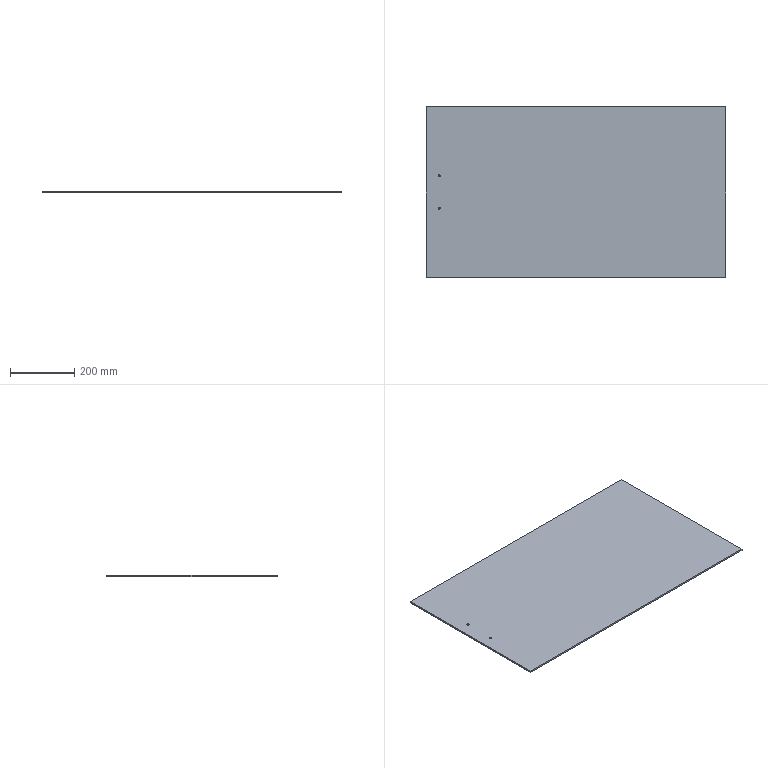Part | SolidWorks | features MirrorStock 1 | 1 solid | 10 faces | box 930 x 530 x 5 mm | volume 2464158 mm3 | plane 6 | cylinder 4 | commonest cylinder face diameters 6.6 x4
STEP:
#1=CARTESIAN_POINT('',(-421.7,50.,-5.));
#2=VERTEX_POINT('',#1);
#3=CARTESIAN_POINT('',(-428.3,50.,-5.));
#4=VERTEX_POINT('',#3);
#5=CARTESIAN_POINT('',(-425.,50.,-5.));
#6=DIRECTION('',(0.,0.,1.));
#7=DIRECTION('',(1.,0.,0.));
#8=AXIS2_PLACEMENT_3D('',#5,#6,#7);
#9=CIRCLE('',#8,3.3);
#10=EDGE_CURVE('',#2,#4,#9,.T.);
#11=ORIENTED_EDGE('',*,*,#10,.F.);
#12=CARTESIAN_POINT('',(-421.7,50.,0.));
#13=VERTEX_POINT('',#12);
#14=CARTESIAN_POINT('',(-421.7,50.,-10.));
#15=DIRECTION('',(0.,0.,1.));
#16=VECTOR('',#15,1000.);
#17=LINE('',#14,#16);
#18=EDGE_CURVE('',#2,#13,#17,.T.);
#19=ORIENTED_EDGE('',*,*,#18,.T.);
#20=CARTESIAN_POINT('',(-428.3,50.,0.));
#21=VERTEX_POINT('',#20);
#22=CARTESIAN_POINT('',(-425.,50.,0.));
#23=DIRECTION('',(0.,0.,-1.));
#24=DIRECTION('',(-1.,0.,0.));
#25=AXIS2_PLACEMENT_3D('',#22,#23,#24);
#26=CIRCLE('',#25,3.3);
#27=EDGE_CURVE('',#21,#13,#26,.T.);
#28=ORIENTED_EDGE('',*,*,#27,.F.);
#29=CARTESIAN_POINT('',(-428.3,50.,-10.));
#30=DIRECTION('',(0.,0.,1.));
#31=VECTOR('',#30,1000.);
#32=LINE('',#29,#31);
#33=EDGE_CURVE('',#4,#21,#32,.T.);
#34=ORIENTED_EDGE('',*,*,#33,.F.);
#35=EDGE_LOOP('',(#11,#19,#28,#34));
#36=FACE_OUTER_BOUND('',#35,.T.);
#37=CARTESIAN_POINT('',(-425.,50.,-10.));
#38=DIRECTION('',(0.,0.,1.));
#39=DIRECTION('',(-1.,0.,0.));
#40=AXIS2_PLACEMENT_3D('',#37,#38,#39);
#41=CYLINDRICAL_SURFACE('',#40,3.3);
#42=ADVANCED_FACE('',(#36),#41,.F.);
#43=CARTESIAN_POINT('',(-421.7,-50.,-5.));
#44=VERTEX_POINT('',#43);
#45=CARTESIAN_POINT('',(-428.3,-50.,-5.));
#46=VERTEX_POINT('',#45);
#47=CARTESIAN_POINT('',(-425.,-50.,-5.));
#48=DIRECTION('',(0.,0.,1.));
#49=DIRECTION('',(1.,0.,0.));
#50=AXIS2_PLACEMENT_3D('',#47,#48,#49);
#51=CIRCLE('',#50,3.3);
#52=EDGE_CURVE('',#44,#46,#51,.T.);
#53=ORIENTED_EDGE('',*,*,#52,.F.);
#54=CARTESIAN_POINT('',(-421.7,-50.,0.));
#55=VERTEX_POINT('',#54);
#56=CARTESIAN_POINT('',(-421.7,-50.,-10.));
#57=DIRECTION('',(0.,0.,1.));
#58=VECTOR('',#57,1000.);
#59=LINE('',#56,#58);
#60=EDGE_CURVE('',#44,#55,#59,.T.);
#61=ORIENTED_EDGE('',*,*,#60,.T.);
#62=CARTESIAN_POINT('',(-428.3,-50.,0.));
#63=VERTEX_POINT('',#62);
#64=CARTESIAN_POINT('',(-425.,-50.,0.));
#65=DIRECTION('',(0.,0.,-1.));
#66=DIRECTION('',(-1.,0.,0.));
#67=AXIS2_PLACEMENT_3D('',#64,#65,#66);
#68=CIRCLE('',#67,3.3);
#69=EDGE_CURVE('',#63,#55,#68,.T.);
#70=ORIENTED_EDGE('',*,*,#69,.F.);
#71=CARTESIAN_POINT('',(-428.3,-50.,-10.));
#72=DIRECTION('',(0.,0.,1.));
#73=VECTOR('',#72,1000.);
#74=LINE('',#71,#73);
#75=EDGE_CURVE('',#46,#63,#74,.T.);
#76=ORIENTED_EDGE('',*,*,#75,.F.);
#77=EDGE_LOOP('',(#53,#61,#70,#76));
#78=FACE_OUTER_BOUND('',#77,.T.);
#79=CARTESIAN_POINT('',(-425.,-50.,-10.));
#80=DIRECTION('',(0.,0.,1.));
#81=DIRECTION('',(-1.,0.,0.));
#82=AXIS2_PLACEMENT_3D('',#79,#80,#81);
#83=CYLINDRICAL_SURFACE('',#82,3.3);
#84=ADVANCED_FACE('',(#78),#83,.F.);
#85=CARTESIAN_POINT('',(-465.,265.,0.));
#86=VERTEX_POINT('',#85);
#87=CARTESIAN_POINT('',(-465.,-265.,0.));
#88=VERTEX_POINT('',#87);
#89=CARTESIAN_POINT('',(-465.,-265.,0.));
#90=DIRECTION('',(0.,-1.,0.));
#91=VECTOR('',#90,1000.);
#92=LINE('',#89,#91);
#93=EDGE_CURVE('',#86,#88,#92,.T.);
#94=ORIENTED_EDGE('',*,*,#93,.F.);
#95=CARTESIAN_POINT('',(-465.,265.,-5.));
#96=VERTEX_POINT('',#95);
#97=CARTESIAN_POINT('',(-465.,265.,-5.));
#98=DIRECTION('',(0.,0.,1.));
#99=VECTOR('',#98,1000.);
#100=LINE('',#97,#99);
#101=EDGE_CURVE('',#96,#86,#100,.T.);
#102=ORIENTED_EDGE('',*,*,#101,.F.);
#103=CARTESIAN_POINT('',(-465.,-265.,-5.));
#104=VERTEX_POINT('',#103);
#105=CARTESIAN_POINT('',(-465.,-265.,-5.));
#106=DIRECTION('',(0.,-1.,0.));
#107=VECTOR('',#106,1000.);
#108=LINE('',#105,#107);
#109=EDGE_CURVE('',#96,#104,#108,.T.);
#110=ORIENTED_EDGE('',*,*,#109,.T.);
#111=CARTESIAN_POINT('',(-465.,-265.,-5.));
#112=DIRECTION('',(0.,0.,1.));
#113=VECTOR('',#112,1000.);
#114=LINE('',#111,#113);
#115=EDGE_CURVE('',#104,#88,#114,.T.);
#116=ORIENTED_EDGE('',*,*,#115,.T.);
#117=EDGE_LOOP('',(#94,#102,#110,#116));
#118=FACE_OUTER_BOUND('',#117,.T.);
#119=CARTESIAN_POINT('',(-465.,-265.,-5.));
#120=DIRECTION('',(1.,0.,0.));
#121=DIRECTION('',(0.,0.,1.));
#122=AXIS2_PLACEMENT_3D('',#119,#120,#121);
#123=PLANE('',#122);
#124=ADVANCED_FACE('',(#118),#123,.F.);
#125=CARTESIAN_POINT('',(465.,-265.,0.));
#126=VERTEX_POINT('',#125);
#127=CARTESIAN_POINT('',(465.,-265.,0.));
#128=DIRECTION('',(1.,0.,0.));
#129=VECTOR('',#128,1000.);
#130=LINE('',#127,#129);
#131=EDGE_CURVE('',#88,#126,#130,.T.);
#132=ORIENTED_EDGE('',*,*,#131,.F.);
#133=ORIENTED_EDGE('',*,*,#115,.F.);
#134=CARTESIAN_POINT('',(465.,-265.,-5.));
#135=VERTEX_POINT('',#134);
#136=CARTESIAN_POINT('',(465.,-265.,-5.));
#137=DIRECTION('',(1.,0.,0.));
#138=VECTOR('',#137,1000.);
#139=LINE('',#136,#138);
#140=EDGE_CURVE('',#104,#135,#139,.T.);
#141=ORIENTED_EDGE('',*,*,#140,.T.);
#142=CARTESIAN_POINT('',(465.,-265.,-5.));
#143=DIRECTION('',(0.,0.,1.));
#144=VECTOR('',#143,1000.);
#145=LINE('',#142,#144);
#146=EDGE_CURVE('',#135,#126,#145,.T.);
#147=ORIENTED_EDGE('',*,*,#146,.T.);
#148=EDGE_LOOP('',(#132,#133,#141,#147));
#149=FACE_OUTER_BOUND('',#148,.T.);
#150=CARTESIAN_POINT('',(465.,-265.,-5.));
#151=DIRECTION('',(0.,1.,0.));
#152=DIRECTION('',(-1.,0.,0.));
#153=AXIS2_PLACEMENT_3D('',#150,#151,#152);
#154=PLANE('',#153);
#155=ADVANCED_FACE('',(#149),#154,.F.);
#156=CARTESIAN_POINT('',(465.,265.,0.));
#157=VERTEX_POINT('',#156);
#158=CARTESIAN_POINT('',(465.,-265.,0.));
#159=DIRECTION('',(0.,1.,0.));
#160=VECTOR('',#159,1000.);
#161=LINE('',#158,#160);
#162=EDGE_CURVE('',#126,#157,#161,.T.);
#163=ORIENTED_EDGE('',*,*,#162,.F.);
#164=ORIENTED_EDGE('',*,*,#146,.F.);
#165=CARTESIAN_POINT('',(465.,265.,-5.));
#166=VERTEX_POINT('',#165);
#167=CARTESIAN_POINT('',(465.,-265.,-5.));
#168=DIRECTION('',(0.,1.,0.));
#169=VECTOR('',#168,1000.);
#170=LINE('',#167,#169);
#171=EDGE_CURVE('',#135,#166,#170,.T.);
#172=ORIENTED_EDGE('',*,*,#171,.T.);
#173=CARTESIAN_POINT('',(465.,265.,-5.));
#174=DIRECTION('',(0.,0.,1.));
#175=VECTOR('',#174,1000.);
#176=LINE('',#173,#175);
#177=EDGE_CURVE('',#166,#157,#176,.T.);
#178=ORIENTED_EDGE('',*,*,#177,.T.);
#179=EDGE_LOOP('',(#163,#164,#172,#178));
#180=FACE_OUTER_BOUND('',#179,.T.);
#181=CARTESIAN_POINT('',(465.,-265.,-5.));
#182=DIRECTION('',(-1.,0.,0.));
#183=DIRECTION('',(0.,0.,-1.));
#184=AXIS2_PLACEMENT_3D('',#181,#182,#183);
#185=PLANE('',#184);
#186=ADVANCED_FACE('',(#180),#185,.F.);
#187=CARTESIAN_POINT('',(465.,265.,0.));
#188=DIRECTION('',(-1.,0.,0.));
#189=VECTOR('',#188,1000.);
#190=LINE('',#187,#189);
#191=EDGE_CURVE('',#157,#86,#190,.T.);
#192=ORIENTED_EDGE('',*,*,#191,.F.);
#193=ORIENTED_EDGE('',*,*,#177,.F.);
#194=CARTESIAN_POINT('',(465.,265.,-5.));
#195=DIRECTION('',(-1.,0.,0.));
#196=VECTOR('',#195,1000.);
#197=LINE('',#194,#196);
#198=EDGE_CURVE('',#166,#96,#197,.T.);
#199=ORIENTED_EDGE('',*,*,#198,.T.);
#200=ORIENTED_EDGE('',*,*,#101,.T.);
#201=EDGE_LOOP('',(#192,#193,#199,#200));
#202=FACE_OUTER_BOUND('',#201,.T.);
#203=CARTESIAN_POINT('',(465.,265.,-5.));
#204=DIRECTION('',(0.,-1.,0.));
#205=DIRECTION('',(1.,0.,0.));
#206=AXIS2_PLACEMENT_3D('',#203,#204,#205);
#207=PLANE('',#206);
#208=ADVANCED_FACE('',(#202),#207,.F.);
#209=CARTESIAN_POINT('',(-425.,50.,-5.));
#210=DIRECTION('',(0.,0.,1.));
#211=DIRECTION('',(1.,0.,0.));
#212=AXIS2_PLACEMENT_3D('',#209,#210,#211);
#213=CIRCLE('',#212,3.3);
#214=EDGE_CURVE('',#4,#2,#213,.T.);
#215=ORIENTED_EDGE('',*,*,#214,.T.);
#216=ORIENTED_EDGE('',*,*,#10,.T.);
#217=EDGE_LOOP('',(#215,#216));
#218=FACE_BOUND('',#217,.T.);
#219=CARTESIAN_POINT('',(-425.,-50.,-5.));
#220=DIRECTION('',(0.,0.,1.));
#221=DIRECTION('',(1.,0.,0.));
#222=AXIS2_PLACEMENT_3D('',#219,#220,#221);
#223=CIRCLE('',#222,3.3);
#224=EDGE_CURVE('',#46,#44,#223,.T.);
#225=ORIENTED_EDGE('',*,*,#224,.T.);
#226=ORIENTED_EDGE('',*,*,#52,.T.);
#227=EDGE_LOOP('',(#225,#226));
#228=FACE_BOUND('',#227,.T.);
#229=ORIENTED_EDGE('',*,*,#109,.F.);
#230=ORIENTED_EDGE('',*,*,#198,.F.);
#231=ORIENTED_EDGE('',*,*,#171,.F.);
#232=ORIENTED_EDGE('',*,*,#140,.F.);
#233=EDGE_LOOP('',(#229,#230,#231,#232));
#234=FACE_OUTER_BOUND('',#233,.T.);
#235=CARTESIAN_POINT('',(0.,0.,-5.));
#236=DIRECTION('',(0.,0.,-1.));
#237=DIRECTION('',(1.,0.,0.));
#238=AXIS2_PLACEMENT_3D('',#235,#236,#237);
#239=PLANE('',#238);
#240=ADVANCED_FACE('',(#218,#228,#234),#239,.T.);
#241=ORIENTED_EDGE('',*,*,#27,.T.);
#242=CARTESIAN_POINT('',(-425.,50.,0.));
#243=DIRECTION('',(0.,0.,-1.));
#244=DIRECTION('',(-1.,0.,0.));
#245=AXIS2_PLACEMENT_3D('',#242,#243,#244);
#246=CIRCLE('',#245,3.3);
#247=EDGE_CURVE('',#13,#21,#246,.T.);
#248=ORIENTED_EDGE('',*,*,#247,.T.);
#249=EDGE_LOOP('',(#241,#248));
#250=FACE_BOUND('',#249,.T.);
#251=ORIENTED_EDGE('',*,*,#69,.T.);
#252=CARTESIAN_POINT('',(-425.,-50.,0.));
#253=DIRECTION('',(0.,0.,-1.));
#254=DIRECTION('',(-1.,0.,0.));
#255=AXIS2_PLACEMENT_3D('',#252,#253,#254);
#256=CIRCLE('',#255,3.3);
#257=EDGE_CURVE('',#55,#63,#256,.T.);
#258=ORIENTED_EDGE('',*,*,#257,.T.);
#259=EDGE_LOOP('',(#251,#258));
#260=FACE_BOUND('',#259,.T.);
#261=ORIENTED_EDGE('',*,*,#93,.T.);
#262=ORIENTED_EDGE('',*,*,#131,.T.);
#263=ORIENTED_EDGE('',*,*,#162,.T.);
#264=ORIENTED_EDGE('',*,*,#191,.T.);
#265=EDGE_LOOP('',(#261,#262,#263,#264));
#266=FACE_OUTER_BOUND('',#265,.T.);
#267=CARTESIAN_POINT('',(0.,0.,0.));
#268=DIRECTION('',(0.,0.,-1.));
#269=DIRECTION('',(1.,0.,0.));
#270=AXIS2_PLACEMENT_3D('',#267,#268,#269);
#271=PLANE('',#270);
#272=ADVANCED_FACE('',(#250,#260,#266),#271,.F.);
#273=ORIENTED_EDGE('',*,*,#60,.F.);
#274=ORIENTED_EDGE('',*,*,#224,.F.);
#275=ORIENTED_EDGE('',*,*,#75,.T.);
#276=ORIENTED_EDGE('',*,*,#257,.F.);
#277=EDGE_LOOP('',(#273,#274,#275,#276));
#278=FACE_OUTER_BOUND('',#277,.T.);
#279=CARTESIAN_POINT('',(-425.,-50.,-10.));
#280=DIRECTION('',(0.,0.,1.));
#281=DIRECTION('',(-1.,0.,0.));
#282=AXIS2_PLACEMENT_3D('',#279,#280,#281);
#283=CYLINDRICAL_SURFACE('',#282,3.3);
#284=ADVANCED_FACE('',(#278),#283,.F.);
#285=ORIENTED_EDGE('',*,*,#18,.F.);
#286=ORIENTED_EDGE('',*,*,#214,.F.);
#287=ORIENTED_EDGE('',*,*,#33,.T.);
#288=ORIENTED_EDGE('',*,*,#247,.F.);
#289=EDGE_LOOP('',(#285,#286,#287,#288));
#290=FACE_OUTER_BOUND('',#289,.T.);
#291=CARTESIAN_POINT('',(-425.,50.,-10.));
#292=DIRECTION('',(0.,0.,1.));
#293=DIRECTION('',(-1.,0.,0.));
#294=AXIS2_PLACEMENT_3D('',#291,#292,#293);
#295=CYLINDRICAL_SURFACE('',#294,3.3);
#296=ADVANCED_FACE('',(#290),#295,.F.);
#297=CLOSED_SHELL('',(#42,#84,#124,#155,#186,#208,#240,#272,#284,#296));
#298=MANIFOLD_SOLID_BREP('',#297);
#299=CARTESIAN_POINT('',(0.,0.,0.));
#300=DIRECTION('',(0.,0.,1.));
#301=DIRECTION('',(1.,0.,0.));
#302=AXIS2_PLACEMENT_3D('',#299,#300,#301);
#303=(LENGTH_UNIT()NAMED_UNIT(*)SI_UNIT(.MILLI.,.METRE.));
#304=UNCERTAINTY_MEASURE_WITH_UNIT(LENGTH_MEASURE(0.00001),#303,'','');
#305=(NAMED_UNIT(*)PLANE_ANGLE_UNIT()SI_UNIT($,.RADIAN.));
#306=(NAMED_UNIT(*)SI_UNIT($,.STERADIAN.)SOLID_ANGLE_UNIT());
#307=(GEOMETRIC_REPRESENTATION_CONTEXT(3)GLOBAL_UNCERTAINTY_ASSIGNED_CONTEXT((#304))GLOBAL_UNIT_ASSIGNED_CONTEXT((#303,#305,#306))REPRESENTATION_CONTEXT('',''));
#308=ADVANCED_BREP_SHAPE_REPRESENTATION('',(#298,#302),#307);